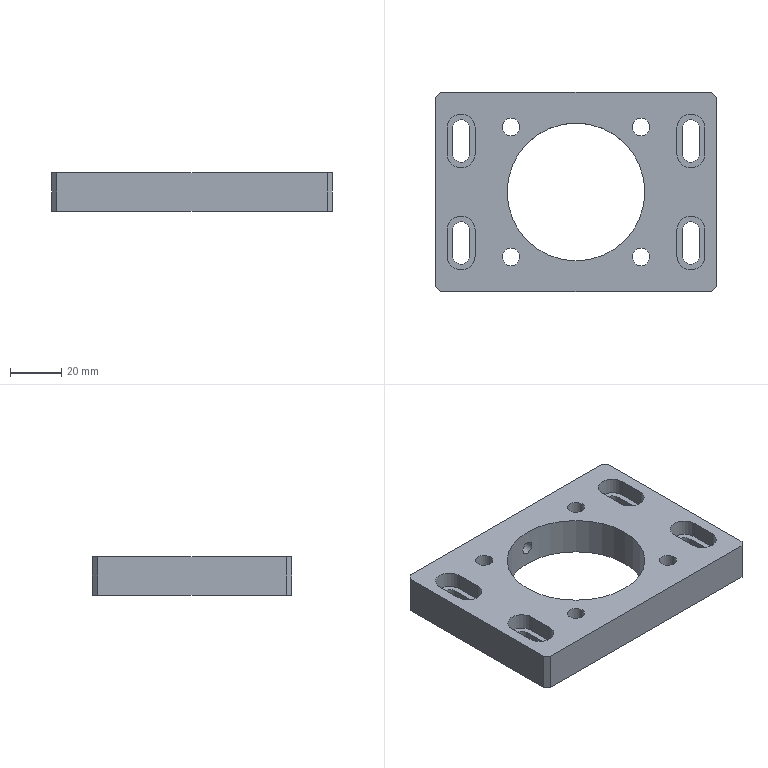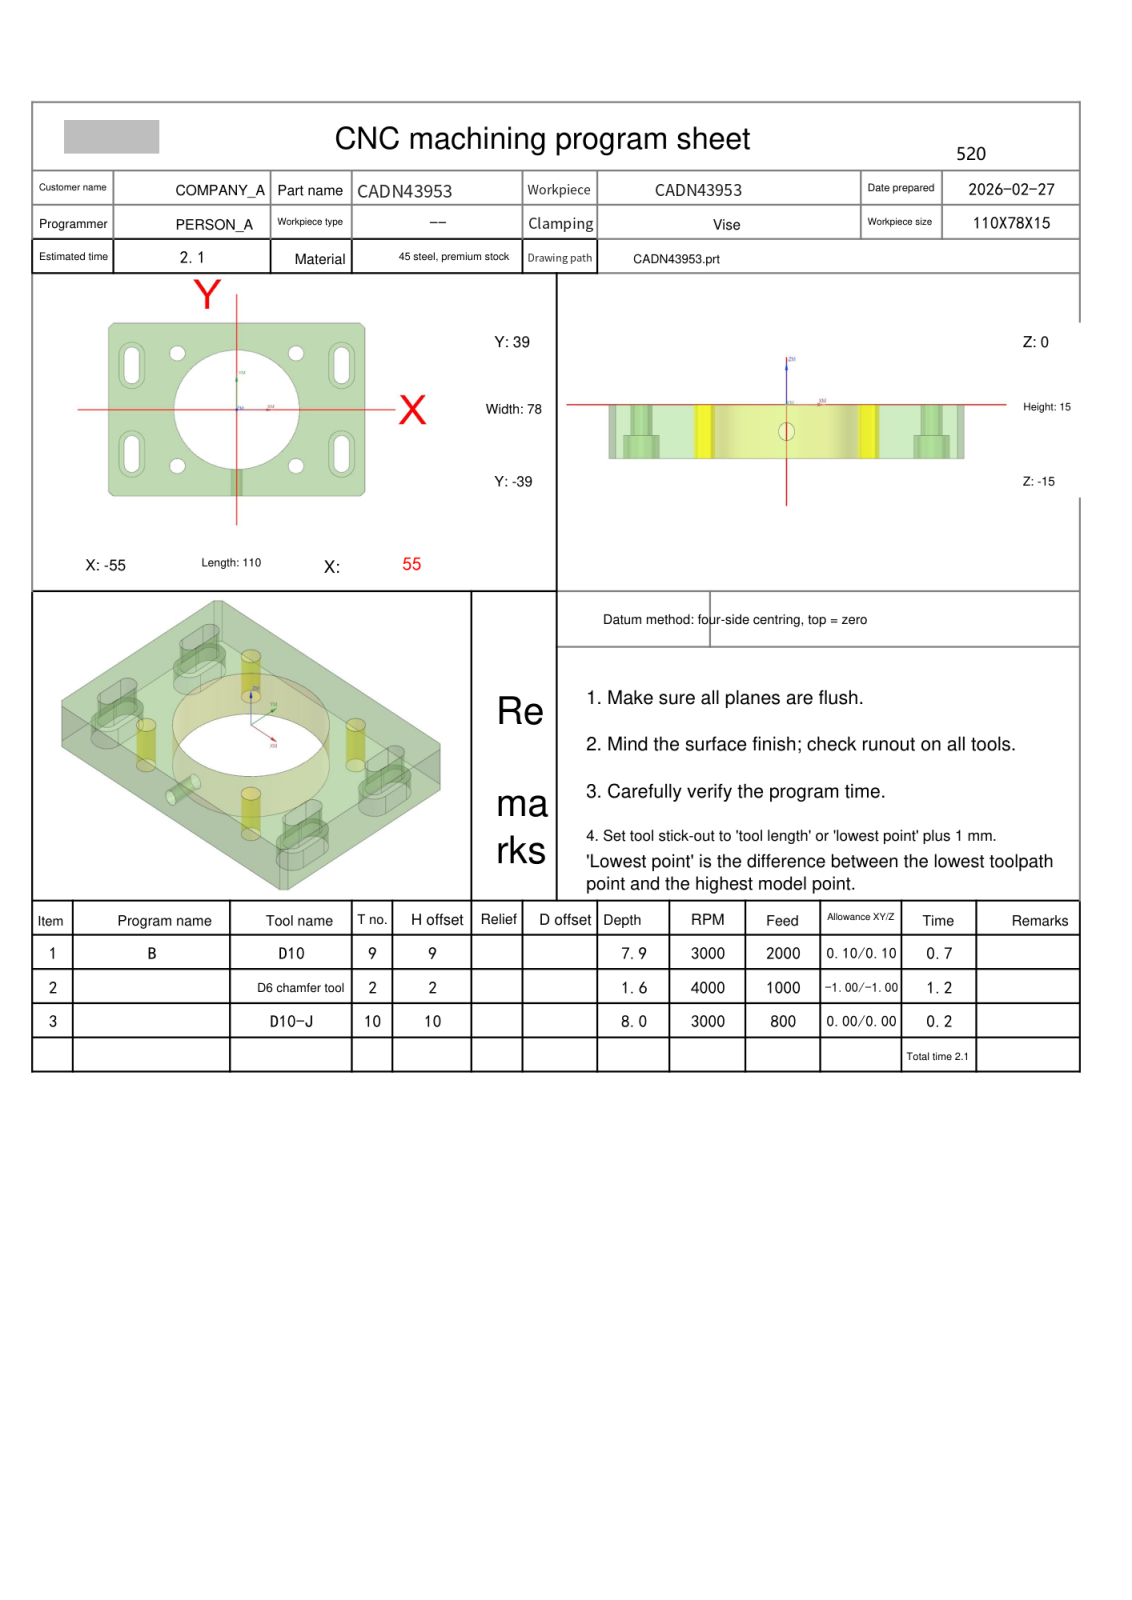NC program | NX | posted by the shop | part box 110 x 78 x 15 mm
Whole program:
%
O0001
(Machine time: 2.64 MIN)
(===Total Tool:3===)
(T9=D10     D=10.  R=0.   D-  H09 Z=-7.9  )
(T2=D6 chamfer tool   D=6.   R=0.   D-  H02 Z=-1.6  )
(T10=D10-J  D=10.  R=0.   D-  H10 Z=-8.   )
G80 G90 G17 G49 G40
G91 G28 Z0
M01
N1 T09 M06
(D10  D=10. R=0. H=09 ce=0.10 di=0.10)
G00 G90 G54 X50.242 Y48.97 M03 S3000
G43 H09 Z50.
M08
Z-.5
G01 X56.606 Y42.606 F2000.
X58.606 Y40.606
X64.97 Y34.242
G00 Z-1.
G01 X58.606 Y40.606
X56.606 Y42.606
X50.242 Y48.97
G00 Z-1.5
G01 X56.606 Y42.606
X58.606 Y40.606
X64.97 Y34.242
G00 Z-2.
G01 X58.606 Y40.606
X56.606 Y42.606
X50.242 Y48.97
G00 Z-2.5
G01 X56.606 Y42.606
X58.606 Y40.606
X64.97 Y34.242
G00 Z-3.
G01 X58.606 Y40.606
X56.606 Y42.606
X50.242 Y48.97
G00 Z-3.5
G01 X56.606 Y42.606
X58.606 Y40.606
X64.97 Y34.242
G00 Z-4.
G01 X58.606 Y40.606
X56.606 Y42.606
X50.242 Y48.97
G00 Z-4.5
G01 X56.606 Y42.606
X58.606 Y40.606
X64.97 Y34.242
G00 Z-5.
G01 X58.606 Y40.606
X56.606 Y42.606
X50.242 Y48.97
G00 Z-5.5
G01 X56.606 Y42.606
X58.606 Y40.606
X64.97 Y34.242
G00 Z-6.
G01 X58.606 Y40.606
X56.606 Y42.606
X50.242 Y48.97
G00 Z-6.5
G01 X56.606 Y42.606
X58.606 Y40.606
X64.97 Y34.242
G00 Z-7.
G01 X58.606 Y40.606
X56.606 Y42.606
X50.242 Y48.97
G00 Z-7.5
G01 X56.606 Y42.606
X58.606 Y40.606
X64.97 Y34.242
G00 Z-7.9
G01 X58.606 Y40.606
X56.606 Y42.606
X50.242 Y48.97
G00 Z50.
X64.97 Y-34.242
Z-.5
G01 X58.606 Y-40.606
X56.606 Y-42.606
X50.242 Y-48.97
G00 Z-1.
G01 X56.606 Y-42.606
X58.606 Y-40.606
X64.97 Y-34.242
G00 Z-1.5
G01 X58.606 Y-40.606
X56.606 Y-42.606
X50.242 Y-48.97
G00 Z-2.
G01 X56.606 Y-42.606
X58.606 Y-40.606
X64.97 Y-34.242
G00 Z-2.5
G01 X58.606 Y-40.606
X56.606 Y-42.606
X50.242 Y-48.97
G00 Z-3.
G01 X56.606 Y-42.606
X58.606 Y-40.606
X64.97 Y-34.242
G00 Z-3.5
G01 X58.606 Y-40.606
X56.606 Y-42.606
X50.242 Y-48.97
G00 Z-4.
G01 X56.606 Y-42.606
X58.606 Y-40.606
X64.97 Y-34.242
G00 Z-4.5
G01 X58.606 Y-40.606
X56.606 Y-42.606
X50.242 Y-48.97
G00 Z-5.
G01 X56.606 Y-42.606
X58.606 Y-40.606
X64.97 Y-34.242
G00 Z-5.5
G01 X58.606 Y-40.606
X56.606 Y-42.606
X50.242 Y-48.97
G00 Z-6.
G01 X56.606 Y-42.606
X58.606 Y-40.606
X64.97 Y-34.242
G00 Z-6.5
G01 X58.606 Y-40.606
X56.606 Y-42.606
X50.242 Y-48.97
G00 Z-7.
G01 X56.606 Y-42.606
X58.606 Y-40.606
X64.97 Y-34.242
G00 Z-7.5
G01 X58.606 Y-40.606
X56.606 Y-42.606
X50.242 Y-48.97
G00 Z-7.9
G01 X56.606 Y-42.606
X58.606 Y-40.606
X64.97 Y-34.242
G00 Z50.
X-50.242 Y-48.97
Z-.5
G01 X-56.606 Y-42.606
X-58.606 Y-40.606
X-64.97 Y-34.242
G00 Z-1.
G01 X-58.606 Y-40.606
X-56.606 Y-42.606
X-50.242 Y-48.97
G00 Z-1.5
G01 X-56.606 Y-42.606
X-58.606 Y-40.606
X-64.97 Y-34.242
G00 Z-2.
G01 X-58.606 Y-40.606
X-56.606 Y-42.606
X-50.242 Y-48.97
G00 Z-2.5
G01 X-56.606 Y-42.606
X-58.606 Y-40.606
X-64.97 Y-34.242
G00 Z-3.
G01 X-58.606 Y-40.606
X-56.606 Y-42.606
X-50.242 Y-48.97
G00 Z-3.5
G01 X-56.606 Y-42.606
X-58.606 Y-40.606
X-64.97 Y-34.242
G00 Z-4.
G01 X-58.606 Y-40.606
X-56.606 Y-42.606
X-50.242 Y-48.97
G00 Z-4.5
G01 X-56.606 Y-42.606
X-58.606 Y-40.606
X-64.97 Y-34.242
G00 Z-5.
G01 X-58.606 Y-40.606
X-56.606 Y-42.606
X-50.242 Y-48.97
G00 Z-5.5
G01 X-56.606 Y-42.606
X-58.606 Y-40.606
X-64.97 Y-34.242
G00 Z-6.
G01 X-58.606 Y-40.606
X-56.606 Y-42.606
X-50.242 Y-48.97
G00 Z-6.5
G01 X-56.606 Y-42.606
X-58.606 Y-40.606
X-64.97 Y-34.242
G00 Z-7.
G01 X-58.606 Y-40.606
X-56.606 Y-42.606
X-50.242 Y-48.97
G00 Z-7.5
G01 X-56.606 Y-42.606
X-58.606 Y-40.606
X-64.97 Y-34.242
G00 Z-7.9
G01 X-58.606 Y-40.606
X-56.606 Y-42.606
X-50.242 Y-48.97
G00 Z50.
X-64.97 Y34.242
Z-.5
G01 X-58.606 Y40.606
X-56.606 Y42.606
X-50.242 Y48.97
G00 Z-1.
G01 X-56.606 Y42.606
X-58.606 Y40.606
X-64.97 Y34.242
G00 Z-1.5
G01 X-58.606 Y40.606
X-56.606 Y42.606
X-50.242 Y48.97
G00 Z-2.
G01 X-56.606 Y42.606
X-58.606 Y40.606
X-64.97 Y34.242
G00 Z-2.5
G01 X-58.606 Y40.606
X-56.606 Y42.606
X-50.242 Y48.97
G00 Z-3.
G01 X-56.606 Y42.606
X-58.606 Y40.606
X-64.97 Y34.242
G00 Z-3.5
G01 X-58.606 Y40.606
X-56.606 Y42.606
X-50.242 Y48.97
G00 Z-4.
G01 X-56.606 Y42.606
X-58.606 Y40.606
X-64.97 Y34.242
G00 Z-4.5
G01 X-58.606 Y40.606
X-56.606 Y42.606
X-50.242 Y48.97
G00 Z-5.
G01 X-56.606 Y42.606
X-58.606 Y40.606
X-64.97 Y34.242
G00 Z-5.5
G01 X-58.606 Y40.606
X-56.606 Y42.606
X-50.242 Y48.97
G00 Z-6.
G01 X-56.606 Y42.606
X-58.606 Y40.606
X-64.97 Y34.242
G00 Z-6.5
G01 X-58.606 Y40.606
X-56.606 Y42.606
X-50.242 Y48.97
G00 Z-7.
G01 X-56.606 Y42.606
X-58.606 Y40.606
X-64.97 Y34.242
G00 Z-7.5
G01 X-58.606 Y40.606
X-56.606 Y42.606
X-50.242 Y48.97
G00 Z-7.9
G01 X-56.606 Y42.606
X-58.606 Y40.606
X-64.97 Y34.242
G00 Z50.
G91 G28 Z0.0
M05
M09
G91 G28 Z0.0
M01
N2 T02 M06
(D6 chamfer tool  D=6. R=0. H=02 ce=-1.00 di=-0.80)
G00 G90 G54 X24.461 Y26.956 M03 S4000
G43 H02 Z50.
M08
Z-1.1
G01 Z-1.6 F300.
X24.156
G03 X22.656 Y25.456 I0.0 J-1.5
X25.456 Y22.656 I2.8 J0.0
X28.256 Y25.456 I0.0 J2.8
X25.456 Y28.256 I-2.8 J0.0
X22.656 Y25.456 I0.0 J-2.8
X24.156 Y23.956 I1.5 J0.0
G01 X24.461
Z-1.1
G00 Z50.
X-26.451 Y26.956
Z-1.1
G01 Z-1.6
X-26.756
G03 X-28.256 Y25.456 I0.0 J-1.5
X-25.456 Y22.656 I2.8 J0.0
X-22.656 Y25.456 I0.0 J2.8
X-25.456 Y28.256 I-2.8 J0.0
X-28.256 Y25.456 I0.0 J-2.8
X-26.756 Y23.956 I1.5 J0.0
G01 X-26.451
Z-1.1
G00 Z50.
Y-23.956
Z-1.1
G01 Z-1.6
X-26.756
G03 X-28.256 Y-25.456 I0.0 J-1.5
X-25.456 Y-28.256 I2.8 J0.0
X-22.656 Y-25.456 I0.0 J2.8
X-25.456 Y-22.656 I-2.8 J0.0
X-28.256 Y-25.456 I0.0 J-2.8
X-26.756 Y-26.956 I1.5 J0.0
G01 X-26.451
Z-1.1
G00 Z50.
X24.461 Y-23.956
Z-1.1
G01 Z-1.6
X24.156
G03 X22.656 Y-25.456 I0.0 J-1.5
X25.456 Y-28.256 I2.8 J0.0
X28.256 Y-25.456 I0.0 J2.8
X25.456 Y-22.656 I-2.8 J0.0
X22.656 Y-25.456 I0.0 J-2.8
X24.156 Y-26.956 I1.5 J0.0
G01 X24.461
Z-1.1
G00 Z50.
G00 G90 X-.386 Y40.227 M03 S3500
Z50.
Z.172
G01 Z-1.2 F1000.
G03 X-.1 Y40.027 I1.286 J1.532
G01 X-.054 Y39.997
X0.0 Y40.
X53.
X53.259 Y39.966
X53.5 Y39.866
X53.707 Y39.707
X55.707 Y37.707
X55.866 Y37.5
X55.966 Y37.259
X56. Y37.
Y-37.
X55.966 Y-37.259
X55.866 Y-37.5
X55.707 Y-37.707
X53.707 Y-39.707
X53.5 Y-39.866
X53.259 Y-39.966
X53. Y-40.
X-53.
X-53.259 Y-39.966
X-53.5 Y-39.866
X-53.707 Y-39.707
X-55.707 Y-37.707
X-55.866 Y-37.5
X-55.966 Y-37.259
X-56. Y-37.
Y37.
X-55.966 Y37.259
X-55.866 Y37.5
X-55.707 Y37.707
X-53.707 Y39.707
X-53.5 Y39.866
X-53.259 Y39.966
X-53. Y40.
X0.0
X.054 Y39.997
X.1 Y40.027
G03 X.386 Y40.227 I-1. J1.732
G01 Z.172
G00 Z10.
X42.927 Y20.386
Z.172
G01 Z-1.2
G03 X42.727 Y20.1 I1.532 J-1.286
G01 X42.697 Y20.054
X42.7 Y20.
Y15.
G03 X45. Y12.7 I2.3 J0.0
X47.3 Y15. I0.0 J2.3
G01 Y25.
G03 X45. Y27.3 I-2.3 J0.0
X42.7 Y25. I0.0 J-2.3
G01 Y20.
X42.697 Y19.946
X42.727 Y19.9
G03 X42.927 Y19.614 I1.732 J1.
G01 Z.172
G00 Z10.
X23.248 Y25.86
Z.252
G01 Z-1.2
G03 X23.074 Y25.558 I1.638 J-1.147
G01 X23.048 Y25.51
X23.056 Y25.456
G03 X25.456 Y23.056 I2.4 J0.0
X27.856 Y25.456 I0.0 J2.4
X25.456 Y27.856 I-2.4 J0.0
X23.056 Y25.456 I0.0 J-2.4
G01 X23.048 Y25.402
X23.074 Y25.354
G03 X23.248 Y25.052 I1.813 J.845
G01 Z.252
G00 Z10.
X42.927 Y-19.614
Z.172
G01 Z-1.2
G03 X42.727 Y-19.9 I1.532 J-1.286
G01 X42.697 Y-19.946
X42.7 Y-20.
Y-25.
G03 X45. Y-27.3 I2.3 J0.0
X47.3 Y-25. I0.0 J2.3
G01 Y-15.
G03 X45. Y-12.7 I-2.3 J0.0
X42.7 Y-15. I0.0 J-2.3
G01 Y-20.
X42.697 Y-20.054
X42.727 Y-20.1
G03 X42.927 Y-20.386 I1.732 J1.
G01 Z.172
G00 Z10.
X23.248 Y-25.052
Z.252
G01 Z-1.2
G03 X23.074 Y-25.354 I1.638 J-1.147
G01 X23.048 Y-25.402
X23.056 Y-25.456
G03 X25.456 Y-27.856 I2.4 J0.0
X27.856 Y-25.456 I0.0 J2.4
X25.456 Y-23.056 I-2.4 J0.0
X23.056 Y-25.456 I0.0 J-2.4
G01 X23.048 Y-25.51
X23.074 Y-25.558
G03 X23.248 Y-25.86 I1.813 J.845
G01 Z.252
G00 Z10.
X-25.784 Y.392
Z.194
G01 Z-1.2
G03 X-25.976 Y.101 I1.567 J-1.243
G01 X-26.004 Y.054
X-26. Y0.0
G03 X0.0 Y-26. I26. J0.0
X26. Y0.0 I0.0 J26.
X0.0 Y26. I-26. J0.0
X-26. Y0.0 I0.0 J-26.
G01 X-26.004 Y-.054
X-25.976 Y-.101
G03 X-25.784 Y-.392 I1.759 J.952
G01 Z.194
G00 Z10.
X-27.664 Y25.86
Z.252
G01 Z-1.2
G03 X-27.838 Y25.558 I1.638 J-1.147
G01 X-27.863 Y25.51
X-27.856 Y25.456
G03 X-25.456 Y23.056 I2.4 J0.0
X-23.056 Y25.456 I0.0 J2.4
X-25.456 Y27.856 I-2.4 J0.0
X-27.856 Y25.456 I0.0 J-2.4
G01 X-27.863 Y25.402
X-27.838 Y25.354
G03 X-27.664 Y25.052 I1.813 J.845
G01 Z.252
G00 Z10.
X-42.927 Y19.614
Z.172
G01 Z-1.2
G03 X-42.727 Y19.9 I-1.532 J1.286
G01 X-42.697 Y19.946
X-42.7 Y20.
Y25.
G03 X-45. Y27.3 I-2.3 J0.0
X-47.3 Y25. I0.0 J-2.3
G01 Y15.
G03 X-45. Y12.7 I2.3 J0.0
X-42.7 Y15. I0.0 J2.3
G01 Y20.
X-42.697 Y20.054
X-42.727 Y20.1
G03 X-42.927 Y20.386 I-1.732 J-1.
G01 Z.172
G00 Z10.
Y-20.386
Z.172
G01 Z-1.2
G03 X-42.727 Y-20.1 I-1.532 J1.286
G01 X-42.697 Y-20.054
X-42.7 Y-20.
Y-15.
G03 X-45. Y-12.7 I-2.3 J0.0
X-47.3 Y-15. I0.0 J-2.3
G01 Y-25.
G03 X-45. Y-27.3 I2.3 J0.0
X-42.7 Y-25. I0.0 J2.3
G01 Y-20.
X-42.697 Y-19.946
X-42.727 Y-19.9
G03 X-42.927 Y-19.614 I-1.732 J-1.
G01 Z.172
G00 Z10.
X-27.664 Y-25.052
Z.252
G01 Z-1.2
G03 X-27.838 Y-25.354 I1.638 J-1.147
G01 X-27.863 Y-25.402
X-27.856 Y-25.456
G03 X-25.456 Y-27.856 I2.4 J0.0
X-23.056 Y-25.456 I0.0 J2.4
X-25.456 Y-23.056 I-2.4 J0.0
X-27.856 Y-25.456 I0.0 J-2.4
G01 X-27.863 Y-25.51
X-27.838 Y-25.558
G03 X-27.664 Y-25.86 I1.813 J.845
G01 Z.252
G00 Z50.
G91 G28 Z0.0
M05
M09
G91 G28 Z0.0
M01
N3 T10 M06
(D10-J  D=10. R=0. H=10 ce=0.00 di=0.00)
G00 G90 G54 X52.293 Y46.778 M03 S3000
G43 H10 Z50.
M08
Z-7.
G01 Z-8. F800.
X56.536 Y42.536
X58.536 Y40.536
X62.778 Y36.293
Z-7.
G00 Z50.
Y-36.293
Z-7.
G01 Z-8.
X58.536 Y-40.536
X56.536 Y-42.536
X52.293 Y-46.778
Z-7.
G00 Z50.
X-52.293
Z-7.
G01 Z-8.
X-56.536 Y-42.536
X-58.536 Y-40.536
X-62.778 Y-36.293
Z-7.
G00 Z50.
Y36.293
Z-7.
G01 Z-8.
X-58.536 Y40.536
X-56.536 Y42.536
X-52.293 Y46.778
Z-7.
G00 Z50.
M05
M09
G91 G28 Z0.0
G91 G28 Y0.0
M30
%